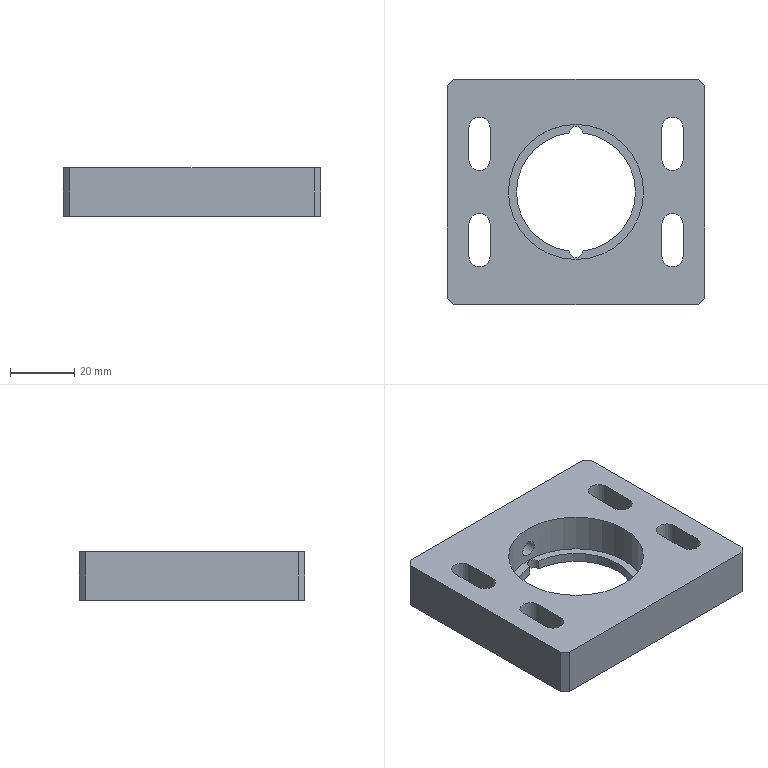Part | 1 solid | 61 faces | box 80 x 70 x 15 mm | volume 54866 mm3 | plane 31 | cylinder 26 | cone 4 | commonest cylinder face diameters 6.6 x8 11 x8 2.5 x4 4 x2 37 x2 5 x1